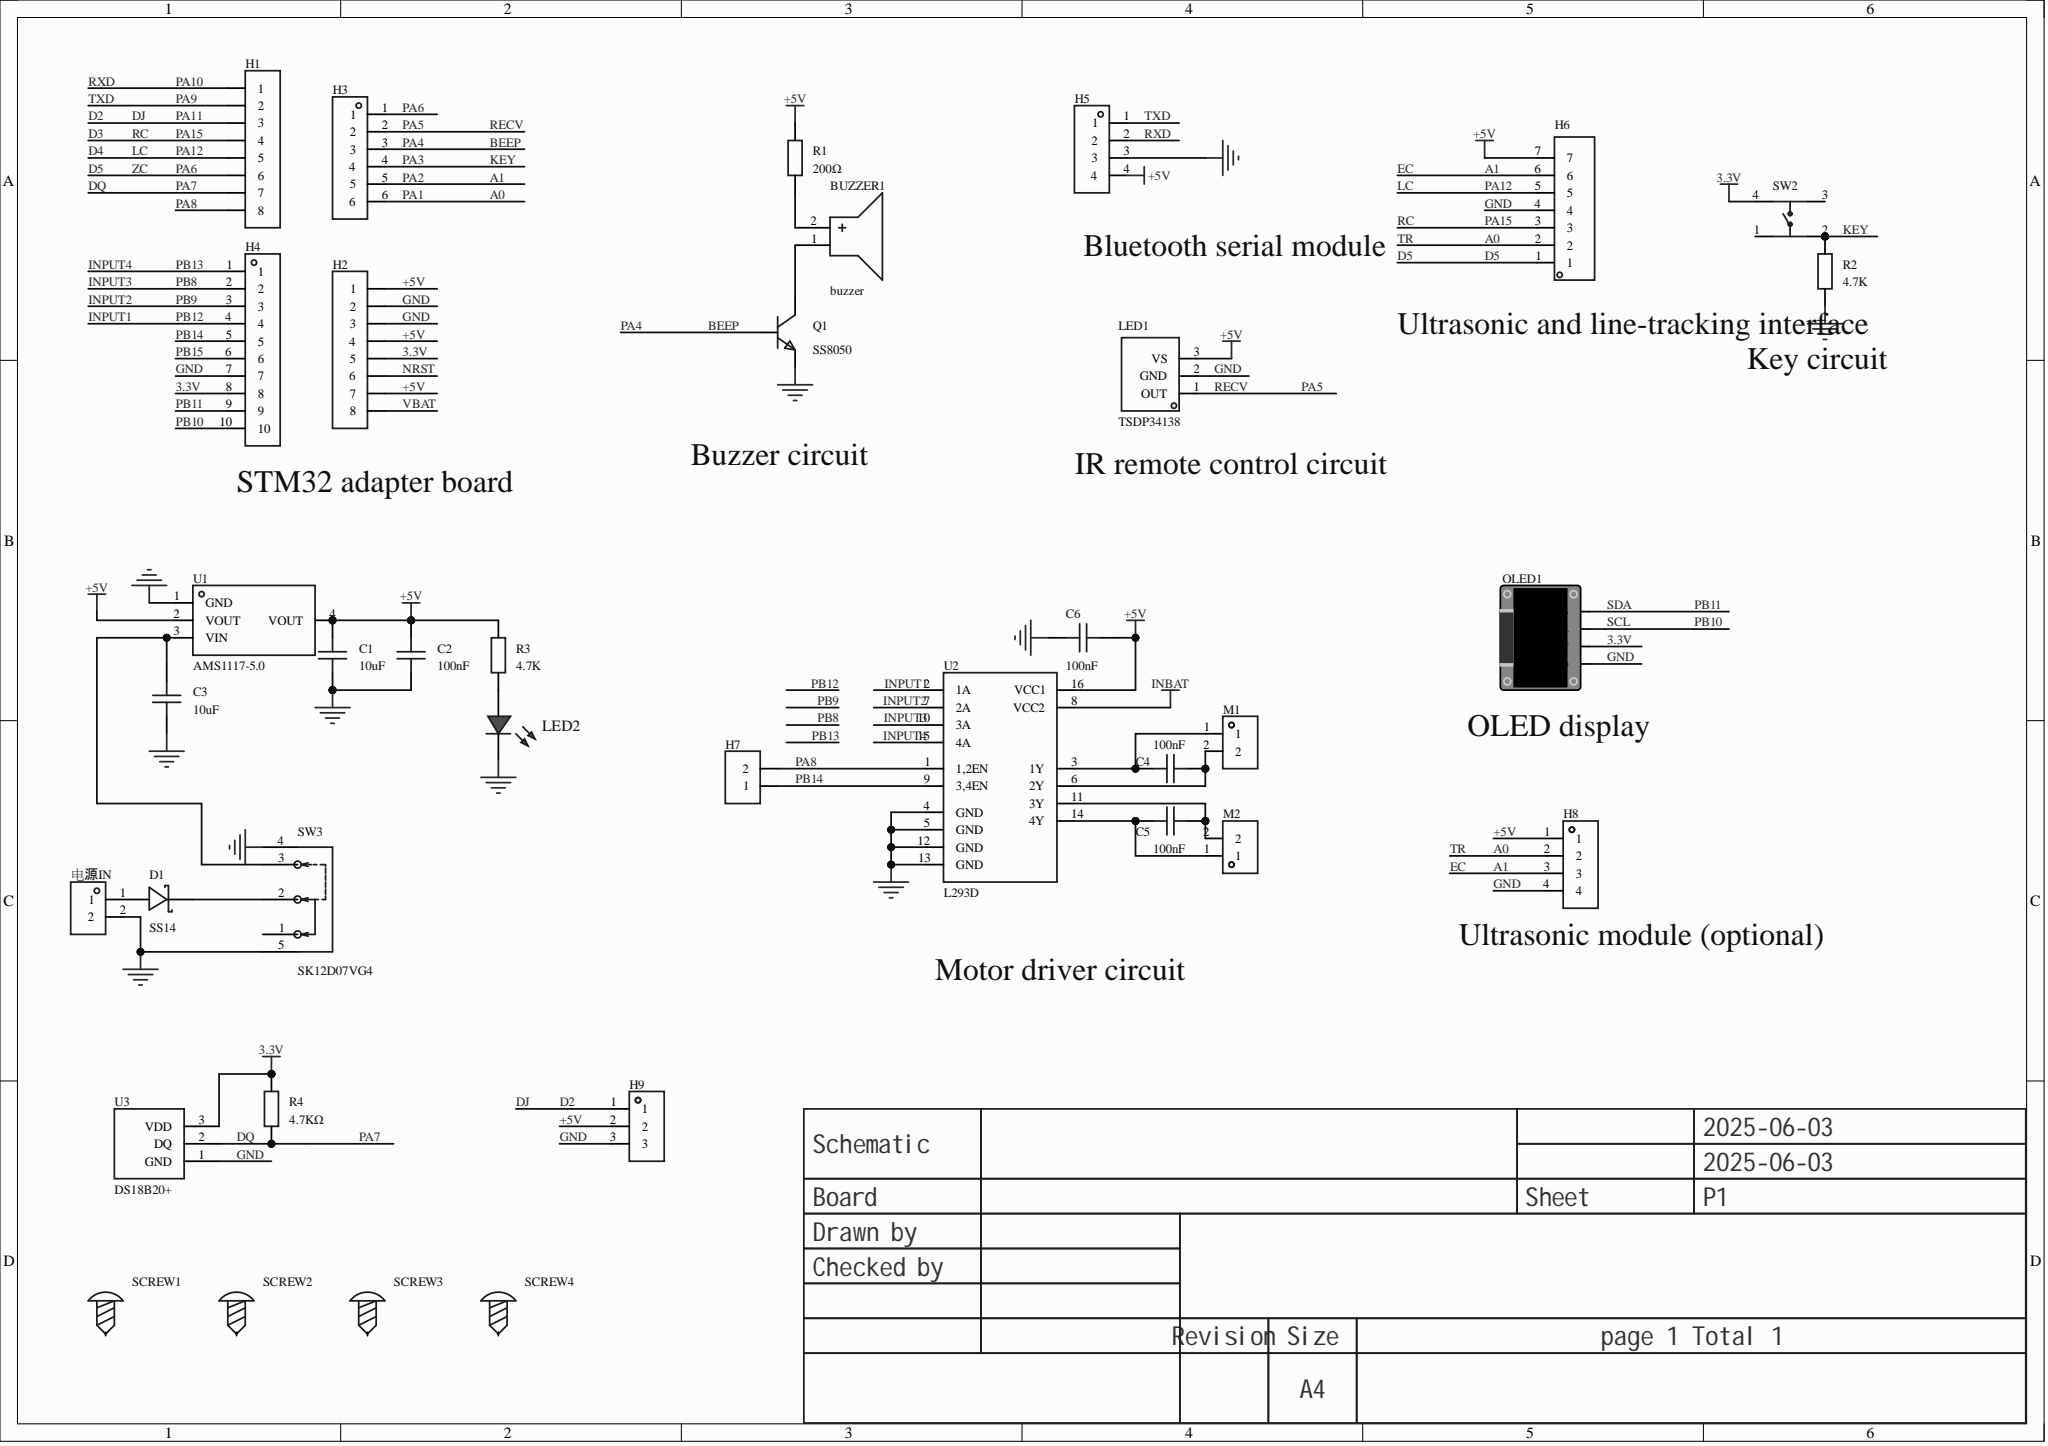Circuit board | Altium Designer | 37 parts | 33 nets
Bill of materials:
Comment,Description,Designator,Footprint,LibRef,Quantity
"buzzer","","BUZZER1","BUZ-TH_BD12.0-P6.00-D0.9-RD","buzzer","1"
"10uF","","C1, C3","C0805","CAP_0805","2"
"100nF","","C2, C4, C5, C6","C0805","CAP_0805","4"
"SS14","Diode configuration: single; forward voltage (Vf): 550mV@1A; DC reverse voltage (Vr): 40V; rectifier current: 1A;","D1","SMA_L4.2-W2.6-LS5.3-RD","SS14_C2480","1"
"","","H1, H2","HDR-TH_8P-P2.54-V-F-1","HDR-F_2.54_1x8P","2"
"","","H3","HDR-TH_6P-P2.54-V-F","HDR-F_2.54_1x6P","1"
"","","H4","HDR-TH_10P-P2.54-V-F","HDR-F_2.54_1x10P","1"
"","","H5, H8","HDR-TH_4P-P2.54-V-F","HDR-F_2.54_1x4P","2"
"","","H6","HDR-TH_7P-P2.54-V-F","HDR-F_2.54_1x7P","1"
"","","H7","HDR-TH_2P-P2.54-V-F","HDR-F_2.54_1x2P","1"
"","","H9","HDR-TH_3P-P2.54-V-M","HDR-M_2.54_1x3P","1"
"TSDP34138","Operating voltage: 2.5V~5.5V; operating current: 350uA; receiving distance: 35m; centre frequency: 38.4kHz; receiving angle: ±45°;","LED1","SENSOR-TH_TSDP34138","TSDP34138","1"
"","","LED2","LED_0603","LED_0603-R","1"
"HX25003-2A","","M1, 电源IN","CONN-TH_2P-P2.50_HX25003-2A","HX25003-2A_C2915012","2"
"HX25003-2A_C2915012","","M2","CONN-TH_2P-P2.50_HX25003-2A","HX25003-2A_C2915012","1"
"","","OLED1","0.96OLED_4P","0.96OLED模块_4P","1"
"SS8050","","Q1","SOT-23-3_L2.9-W1.3-P1.90-LS2.4-BR","SS8050","1"
"200Ω","","R1","R0805","Res_0805","1"
"4.7K","","R2, R3","R0805","Res_0805","2"
"4.7KΩ","","R4","R0805","Res_0805","1"
"","","SCREW1, SCREW2, SCREW3, SCREW4","M3螺丝","M3螺丝","4"
"TS1702-CZ65HBS","","SW2","SW-TH_4P-L6.0-W6.0-P4.50-LS6.3","TS1702-CZ65HBS","1"
"SK12D07VG4","Circuit: single pole double throw; mounting: -; rated current (DC): 500mA; rated voltage (DC): 50V; rated current (AC): -; rated voltage (AC): -; mechanical life: 5千 cycles;","SW3","SW-TH_SK12D07VG4","SK12D07VG4","1"
"AMS1117-5.0","Output type: fixed; operating voltage: 12V; output voltage: 5V; output current: 1A; power supply ripple rejection (PSRR): -; output polarity: positive;","U1","SOT-223_L6.5-W3.5-P2.30-LS7.0-BR","AMS1117-5.0_C6187","1"
"L293D","Push-pull quad-channel driver with diodes","U2","DIP-16_L20.0-W6.4-P2.54-LS7.6-BL","L293D","1"
"DS18B20+","1-Wire digital thermometer with programmable resolution; high-accuracy temperature measurement with minimal wiring, ideal for multi-sensor measurement systems","U3","TO-92-3_L4.9-W3.7-P1.27-L","DS18B20+","1"
Netlist (Protel format):
[
BUZZER1
BUZ-TH_BD12.0-P6.00-D0.9-RD
buzzer



]
[
C1
C0805
10uF



]
[
C2
C0805
100nF



]
[
C3
C0805
10uF



]
[
C4
C0805
100nF



]
[
C5
C0805
100nF



]
[
C6
C0805
100nF



]
[
D1
SMA_L4.2-W2.6-LS5.3-RD
SS14



]
[
H1
HDR-TH_8P-P2.54-V-F-1




]
[
H2
HDR-TH_8P-P2.54-V-F-1




]
[
H3
HDR-TH_6P-P2.54-V-F




]
[
H4
HDR-TH_10P-P2.54-V-F




]
[
H5
HDR-TH_4P-P2.54-V-F




]
[
H6
HDR-TH_7P-P2.54-V-F




]
[
H7
HDR-TH_2P-P2.54-V-F




]
[
H8
HDR-TH_4P-P2.54-V-F




]
[
H9
HDR-TH_3P-P2.54-V-M




]
[
LED1
SENSOR-TH_TSDP34138
TSDP34138



]
[
LED2
LED_0603




]
[
M1
CONN-TH_2P-P2.50_HX25003-2A
HX25003-2A



]
[
M2
CONN-TH_2P-P2.50_HX25003-2A
HX25003-2A_C2915012



]
[
OLED1
0.96OLED_4P




]
[
Q1
SOT-23-3_L2.9-W1.3-P1.90-LS2.4-BR
SS8050



]
[
R1
R0805
200Ω



]
[
R2
R0805
4.7K



]
[
R3
R0805
4.7K



]
[
R4
R0805
4.7KΩ



]
[
SCREW1
M3螺丝




]
[
SCREW2
M3螺丝




]
[
SCREW3
M3螺丝




]
[
SCREW4
M3螺丝




]
[
SW2
SW-TH_4P-L6.0-W6.0-P4.50-LS6.3
TS1702-CZ65HBS



]
[
SW3
SW-TH_SK12D07VG4
SK12D07VG4



]
[
U1
SOT-223_L6.5-W3.5-P2.30-LS7.0-BR
AMS1117-5.0



]
[
U2
DIP-16_L20.0-W6.4-P2.54-LS7.6-BL
L293D



]
[
U3
TO-92-3_L4.9-W3.7-P1.27-L
DS18B20+



]
[
电源IN
CONN-TH_2P-P2.50_HX25003-2A
HX25003-2A



]
(
PB14
H4-5
H7-1
U2-9
)
(
PB11
H4-9
OLED1-4
)
(
PB10
H4-10
OLED1-3
)
(
PA10
H1-1
H5-2
)
(
PA9
H1-2
H5-1
)
(
PA8
H1-8
H7-2
U2-1
)
(
PA5
H3-2
LED1-1
)
(
NetLED2_2
LED2-2
R3-1
)
(
NetD1_2
D1-2
电源IN-1
)
(
NetD1_1
D1-1
SW3-2
)
(
NetC5_2
C5-2
M2-2
U2-11
)
(
NetC5_1
C5-1
M2-1
U2-14
)
(
NetC4_2
C4-2
M1-2
U2-6
)
(
NetC4_1
C4-1
M1-1
U2-3
)
(
NetC3_2
C3-2
SW3-3
U1-3
)
(
NetBUZZER1_2
BUZZER1-2
R1-1
)
(
NetBUZZER1_1
BUZZER1-1
Q1-3
)
(
KEY
H3-4
R2-2
SW2-2
)
(
INPUT4
H4-1
U2-15
)
(
INPUT3
H4-2
U2-10
)
(
INPUT2
H4-3
U2-7
)
(
INPUT1
H4-4
U2-2
)
(
GND
C1-1
C2-1
C3-1
C6-1
H2-2
H2-3
H4-7
H5-3
H6-4
H8-4
H9-3
LED1-2
LED2-1
OLED1-1
Q1-2
R2-1
SW3-4
SW3-5
U1-1
U2-4
U2-5
U2-12
U2-13
U3-1
电源IN-2
)
(
DQ
H1-7
R4-1
U3-2
)
(
D5
H1-6
H3-1
H6-1
)
(
D4
H1-5
H6-5
)
(
D3
H1-4
H6-3
)
(
D2
H1-3
H9-1
)
(
BEEP
H3-3
Q1-1
)
(
A1
H3-5
H6-6
H8-3
)
(
A0
H3-6
H6-2
H8-2
)
(
+5V
C1-2
C2-2
C6-2
H2-1
H2-4
H2-7
H5-4
H6-7
H8-1
H9-2
LED1-3
R1-2
R3-2
U1-2
U1-4
U2-16
)
(
3.3V
H2-5
H4-8
OLED1-2
R4-2
SW2-4
U3-3
)